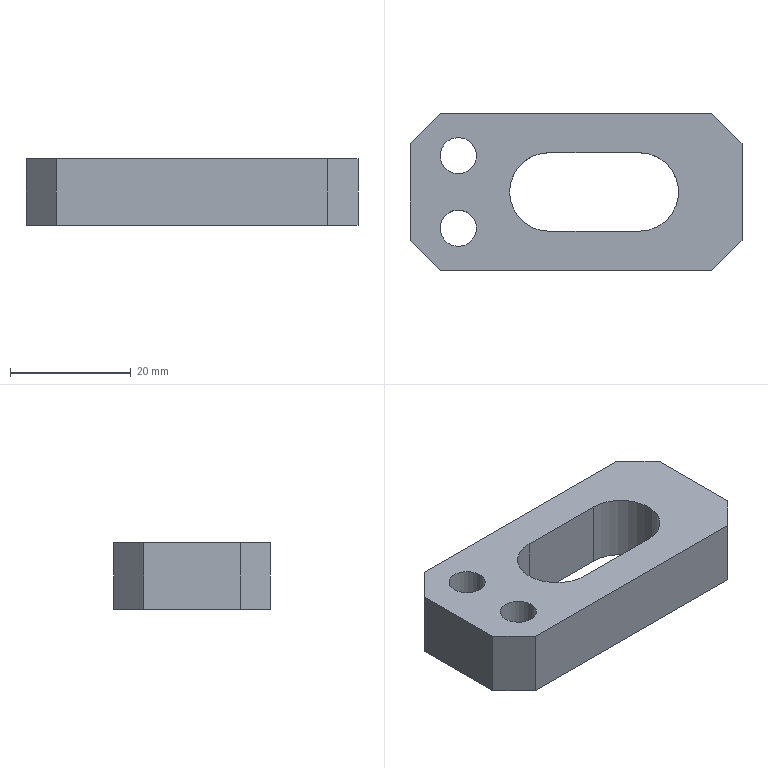Part | SolidWorks | features Chamfer 1, Extrusion 1 | 1 solid | 19 faces | box 55 x 26 x 11 mm | volume 10953 mm3 | plane 12 | cylinder 7 | commonest cylinder face diameters 6 x4 13 x3
STEP:
#1=CARTESIAN_POINT('',(-4.5,6.5,11.));
#2=VERTEX_POINT('',#1);
#3=CARTESIAN_POINT('',(-11.,0.,11.));
#4=VERTEX_POINT('',#3);
#5=CARTESIAN_POINT('',(-4.5,0.,11.));
#6=DIRECTION('',(0.,0.,1.));
#7=DIRECTION('',(1.,0.,0.));
#8=AXIS2_PLACEMENT_3D('',#5,#6,#7);
#9=CIRCLE('',#8,6.5);
#10=EDGE_CURVE('',#2,#4,#9,.T.);
#11=ORIENTED_EDGE('',*,*,#10,.T.);
#12=CARTESIAN_POINT('',(-11.,0.,0.));
#13=VERTEX_POINT('',#12);
#14=CARTESIAN_POINT('',(-11.,0.,11.));
#15=DIRECTION('',(0.,0.,-1.));
#16=VECTOR('',#15,1000.);
#17=LINE('',#14,#16);
#18=EDGE_CURVE('',#4,#13,#17,.T.);
#19=ORIENTED_EDGE('',*,*,#18,.T.);
#20=CARTESIAN_POINT('',(-4.5,6.5,0.));
#21=VERTEX_POINT('',#20);
#22=CARTESIAN_POINT('',(-4.5,0.,0.));
#23=DIRECTION('',(0.,0.,1.));
#24=DIRECTION('',(1.,0.,0.));
#25=AXIS2_PLACEMENT_3D('',#22,#23,#24);
#26=CIRCLE('',#25,6.5);
#27=EDGE_CURVE('',#21,#13,#26,.T.);
#28=ORIENTED_EDGE('',*,*,#27,.F.);
#29=CARTESIAN_POINT('',(-4.5,6.5,11.));
#30=DIRECTION('',(0.,0.,-1.));
#31=VECTOR('',#30,1000.);
#32=LINE('',#29,#31);
#33=EDGE_CURVE('',#2,#21,#32,.T.);
#34=ORIENTED_EDGE('',*,*,#33,.F.);
#35=EDGE_LOOP('',(#11,#19,#28,#34));
#36=FACE_OUTER_BOUND('',#35,.T.);
#37=CARTESIAN_POINT('',(-4.5,0.,11.));
#38=DIRECTION('',(0.,0.,-1.));
#39=DIRECTION('',(-1.,0.,0.));
#40=AXIS2_PLACEMENT_3D('',#37,#38,#39);
#41=CYLINDRICAL_SURFACE('',#40,6.5);
#42=ADVANCED_FACE('',(#36),#41,.F.);
#43=CARTESIAN_POINT('',(-22.5,-6.,11.));
#44=VERTEX_POINT('',#43);
#45=CARTESIAN_POINT('',(-16.5,-6.,11.));
#46=VERTEX_POINT('',#45);
#47=CARTESIAN_POINT('',(-19.5,-6.,11.));
#48=DIRECTION('',(0.,0.,1.));
#49=DIRECTION('',(1.,0.,0.));
#50=AXIS2_PLACEMENT_3D('',#47,#48,#49);
#51=CIRCLE('',#50,3.);
#52=EDGE_CURVE('',#44,#46,#51,.T.);
#53=ORIENTED_EDGE('',*,*,#52,.T.);
#54=CARTESIAN_POINT('',(-16.5,-6.,0.));
#55=VERTEX_POINT('',#54);
#56=CARTESIAN_POINT('',(-16.5,-6.,11.));
#57=DIRECTION('',(0.,0.,-1.));
#58=VECTOR('',#57,1000.);
#59=LINE('',#56,#58);
#60=EDGE_CURVE('',#46,#55,#59,.T.);
#61=ORIENTED_EDGE('',*,*,#60,.T.);
#62=CARTESIAN_POINT('',(-22.5,-6.,0.));
#63=VERTEX_POINT('',#62);
#64=CARTESIAN_POINT('',(-19.5,-6.,0.));
#65=DIRECTION('',(0.,0.,1.));
#66=DIRECTION('',(1.,0.,0.));
#67=AXIS2_PLACEMENT_3D('',#64,#65,#66);
#68=CIRCLE('',#67,3.);
#69=EDGE_CURVE('',#63,#55,#68,.T.);
#70=ORIENTED_EDGE('',*,*,#69,.F.);
#71=CARTESIAN_POINT('',(-22.5,-6.,11.));
#72=DIRECTION('',(0.,0.,-1.));
#73=VECTOR('',#72,1000.);
#74=LINE('',#71,#73);
#75=EDGE_CURVE('',#44,#63,#74,.T.);
#76=ORIENTED_EDGE('',*,*,#75,.F.);
#77=EDGE_LOOP('',(#53,#61,#70,#76));
#78=FACE_OUTER_BOUND('',#77,.T.);
#79=CARTESIAN_POINT('',(-19.5,-6.,11.));
#80=DIRECTION('',(0.,0.,-1.));
#81=DIRECTION('',(-1.,0.,0.));
#82=AXIS2_PLACEMENT_3D('',#79,#80,#81);
#83=CYLINDRICAL_SURFACE('',#82,3.);
#84=ADVANCED_FACE('',(#78),#83,.F.);
#85=CARTESIAN_POINT('',(-22.5,6.,11.));
#86=VERTEX_POINT('',#85);
#87=CARTESIAN_POINT('',(-16.5,6.,11.));
#88=VERTEX_POINT('',#87);
#89=CARTESIAN_POINT('',(-19.5,6.,11.));
#90=DIRECTION('',(0.,0.,1.));
#91=DIRECTION('',(1.,0.,0.));
#92=AXIS2_PLACEMENT_3D('',#89,#90,#91);
#93=CIRCLE('',#92,3.);
#94=EDGE_CURVE('',#86,#88,#93,.T.);
#95=ORIENTED_EDGE('',*,*,#94,.T.);
#96=CARTESIAN_POINT('',(-16.5,6.,0.));
#97=VERTEX_POINT('',#96);
#98=CARTESIAN_POINT('',(-16.5,6.,11.));
#99=DIRECTION('',(0.,0.,-1.));
#100=VECTOR('',#99,1000.);
#101=LINE('',#98,#100);
#102=EDGE_CURVE('',#88,#97,#101,.T.);
#103=ORIENTED_EDGE('',*,*,#102,.T.);
#104=CARTESIAN_POINT('',(-22.5,6.,0.));
#105=VERTEX_POINT('',#104);
#106=CARTESIAN_POINT('',(-19.5,6.,0.));
#107=DIRECTION('',(0.,0.,1.));
#108=DIRECTION('',(1.,0.,0.));
#109=AXIS2_PLACEMENT_3D('',#106,#107,#108);
#110=CIRCLE('',#109,3.);
#111=EDGE_CURVE('',#105,#97,#110,.T.);
#112=ORIENTED_EDGE('',*,*,#111,.F.);
#113=CARTESIAN_POINT('',(-22.5,6.,11.));
#114=DIRECTION('',(0.,0.,-1.));
#115=VECTOR('',#114,1000.);
#116=LINE('',#113,#115);
#117=EDGE_CURVE('',#86,#105,#116,.T.);
#118=ORIENTED_EDGE('',*,*,#117,.F.);
#119=EDGE_LOOP('',(#95,#103,#112,#118));
#120=FACE_OUTER_BOUND('',#119,.T.);
#121=CARTESIAN_POINT('',(-19.5,6.,11.));
#122=DIRECTION('',(0.,0.,-1.));
#123=DIRECTION('',(-1.,0.,0.));
#124=AXIS2_PLACEMENT_3D('',#121,#122,#123);
#125=CYLINDRICAL_SURFACE('',#124,3.);
#126=ADVANCED_FACE('',(#120),#125,.F.);
#127=ORIENTED_EDGE('',*,*,#52,.F.);
#128=CARTESIAN_POINT('',(-19.5,-6.,11.));
#129=DIRECTION('',(0.,0.,1.));
#130=DIRECTION('',(1.,0.,0.));
#131=AXIS2_PLACEMENT_3D('',#128,#129,#130);
#132=CIRCLE('',#131,3.);
#133=EDGE_CURVE('',#46,#44,#132,.T.);
#134=ORIENTED_EDGE('',*,*,#133,.F.);
#135=EDGE_LOOP('',(#127,#134));
#136=FACE_BOUND('',#135,.T.);
#137=ORIENTED_EDGE('',*,*,#94,.F.);
#138=CARTESIAN_POINT('',(-19.5,6.,11.));
#139=DIRECTION('',(0.,0.,1.));
#140=DIRECTION('',(1.,0.,0.));
#141=AXIS2_PLACEMENT_3D('',#138,#139,#140);
#142=CIRCLE('',#141,3.);
#143=EDGE_CURVE('',#88,#86,#142,.T.);
#144=ORIENTED_EDGE('',*,*,#143,.F.);
#145=EDGE_LOOP('',(#137,#144));
#146=FACE_BOUND('',#145,.T.);
#147=CARTESIAN_POINT('',(-22.5,-13.,11.));
#148=VERTEX_POINT('',#147);
#149=CARTESIAN_POINT('',(22.5,-13.,11.));
#150=VERTEX_POINT('',#149);
#151=CARTESIAN_POINT('',(-27.5,-13.,11.));
#152=DIRECTION('',(1.,0.,0.));
#153=VECTOR('',#152,1000.);
#154=LINE('',#151,#153);
#155=EDGE_CURVE('',#148,#150,#154,.T.);
#156=ORIENTED_EDGE('',*,*,#155,.T.);
#157=CARTESIAN_POINT('',(27.5,-8.,11.));
#158=VERTEX_POINT('',#157);
#159=CARTESIAN_POINT('',(27.5,-8.,11.));
#160=DIRECTION('',(0.7071,0.7071,0.));
#161=VECTOR('',#160,1000.);
#162=LINE('',#159,#161);
#163=EDGE_CURVE('',#150,#158,#162,.T.);
#164=ORIENTED_EDGE('',*,*,#163,.T.);
#165=CARTESIAN_POINT('',(27.5,8.,11.));
#166=VERTEX_POINT('',#165);
#167=CARTESIAN_POINT('',(27.5,-13.,11.));
#168=DIRECTION('',(0.,1.,0.));
#169=VECTOR('',#168,1000.);
#170=LINE('',#167,#169);
#171=EDGE_CURVE('',#158,#166,#170,.T.);
#172=ORIENTED_EDGE('',*,*,#171,.T.);
#173=CARTESIAN_POINT('',(22.5,13.,11.));
#174=VERTEX_POINT('',#173);
#175=CARTESIAN_POINT('',(22.5,13.,11.));
#176=DIRECTION('',(-0.7071,0.7071,0.));
#177=VECTOR('',#176,1000.);
#178=LINE('',#175,#177);
#179=EDGE_CURVE('',#166,#174,#178,.T.);
#180=ORIENTED_EDGE('',*,*,#179,.T.);
#181=CARTESIAN_POINT('',(-22.5,13.,11.));
#182=VERTEX_POINT('',#181);
#183=CARTESIAN_POINT('',(-27.5,13.,11.));
#184=DIRECTION('',(-1.,0.,0.));
#185=VECTOR('',#184,1000.);
#186=LINE('',#183,#185);
#187=EDGE_CURVE('',#174,#182,#186,.T.);
#188=ORIENTED_EDGE('',*,*,#187,.T.);
#189=CARTESIAN_POINT('',(-27.5,8.,11.));
#190=VERTEX_POINT('',#189);
#191=CARTESIAN_POINT('',(-27.5,8.,11.));
#192=DIRECTION('',(-0.7071,-0.7071,0.));
#193=VECTOR('',#192,1000.);
#194=LINE('',#191,#193);
#195=EDGE_CURVE('',#182,#190,#194,.T.);
#196=ORIENTED_EDGE('',*,*,#195,.T.);
#197=CARTESIAN_POINT('',(-27.5,-8.,11.));
#198=VERTEX_POINT('',#197);
#199=CARTESIAN_POINT('',(-27.5,-13.,11.));
#200=DIRECTION('',(0.,-1.,0.));
#201=VECTOR('',#200,1000.);
#202=LINE('',#199,#201);
#203=EDGE_CURVE('',#190,#198,#202,.T.);
#204=ORIENTED_EDGE('',*,*,#203,.T.);
#205=CARTESIAN_POINT('',(-22.5,-13.,11.));
#206=DIRECTION('',(0.7071,-0.7071,0.));
#207=VECTOR('',#206,1000.);
#208=LINE('',#205,#207);
#209=EDGE_CURVE('',#198,#148,#208,.T.);
#210=ORIENTED_EDGE('',*,*,#209,.T.);
#211=EDGE_LOOP('',(#156,#164,#172,#180,#188,#196,#204,#210));
#212=FACE_OUTER_BOUND('',#211,.T.);
#213=ORIENTED_EDGE('',*,*,#10,.F.);
#214=CARTESIAN_POINT('',(10.5,6.5,11.));
#215=VERTEX_POINT('',#214);
#216=CARTESIAN_POINT('',(-4.5,6.5,11.));
#217=DIRECTION('',(-1.,0.,0.));
#218=VECTOR('',#217,1000.);
#219=LINE('',#216,#218);
#220=EDGE_CURVE('',#215,#2,#219,.T.);
#221=ORIENTED_EDGE('',*,*,#220,.F.);
#222=CARTESIAN_POINT('',(10.5,-6.5,11.));
#223=VERTEX_POINT('',#222);
#224=CARTESIAN_POINT('',(10.5,0.,11.));
#225=DIRECTION('',(0.,0.,1.));
#226=DIRECTION('',(1.,0.,0.));
#227=AXIS2_PLACEMENT_3D('',#224,#225,#226);
#228=CIRCLE('',#227,6.5);
#229=EDGE_CURVE('',#223,#215,#228,.T.);
#230=ORIENTED_EDGE('',*,*,#229,.F.);
#231=CARTESIAN_POINT('',(-4.5,-6.5,11.));
#232=VERTEX_POINT('',#231);
#233=CARTESIAN_POINT('',(-4.5,-6.5,11.));
#234=DIRECTION('',(1.,0.,0.));
#235=VECTOR('',#234,1000.);
#236=LINE('',#233,#235);
#237=EDGE_CURVE('',#232,#223,#236,.T.);
#238=ORIENTED_EDGE('',*,*,#237,.F.);
#239=CARTESIAN_POINT('',(-4.5,0.,11.));
#240=DIRECTION('',(0.,0.,1.));
#241=DIRECTION('',(1.,0.,0.));
#242=AXIS2_PLACEMENT_3D('',#239,#240,#241);
#243=CIRCLE('',#242,6.5);
#244=EDGE_CURVE('',#4,#232,#243,.T.);
#245=ORIENTED_EDGE('',*,*,#244,.F.);
#246=EDGE_LOOP('',(#213,#221,#230,#238,#245));
#247=FACE_BOUND('',#246,.T.);
#248=CARTESIAN_POINT('',(0.,0.,11.));
#249=DIRECTION('',(0.,0.,-1.));
#250=DIRECTION('',(-1.,0.,0.));
#251=AXIS2_PLACEMENT_3D('',#248,#249,#250);
#252=PLANE('',#251);
#253=ADVANCED_FACE('',(#136,#146,#212,#247),#252,.F.);
#254=ORIENTED_EDGE('',*,*,#111,.T.);
#255=CARTESIAN_POINT('',(-19.5,6.,0.));
#256=DIRECTION('',(0.,0.,1.));
#257=DIRECTION('',(1.,0.,0.));
#258=AXIS2_PLACEMENT_3D('',#255,#256,#257);
#259=CIRCLE('',#258,3.);
#260=EDGE_CURVE('',#97,#105,#259,.T.);
#261=ORIENTED_EDGE('',*,*,#260,.T.);
#262=EDGE_LOOP('',(#254,#261));
#263=FACE_BOUND('',#262,.T.);
#264=CARTESIAN_POINT('',(27.5,-8.,0.));
#265=VERTEX_POINT('',#264);
#266=CARTESIAN_POINT('',(27.5,8.,0.));
#267=VERTEX_POINT('',#266);
#268=CARTESIAN_POINT('',(27.5,-13.,0.));
#269=DIRECTION('',(0.,1.,0.));
#270=VECTOR('',#269,1000.);
#271=LINE('',#268,#270);
#272=EDGE_CURVE('',#265,#267,#271,.T.);
#273=ORIENTED_EDGE('',*,*,#272,.F.);
#274=CARTESIAN_POINT('',(22.5,-13.,0.));
#275=VERTEX_POINT('',#274);
#276=CARTESIAN_POINT('',(17.75,-17.75,0.));
#277=DIRECTION('',(-0.7071,-0.7071,0.));
#278=VECTOR('',#277,1000.);
#279=LINE('',#276,#278);
#280=EDGE_CURVE('',#265,#275,#279,.T.);
#281=ORIENTED_EDGE('',*,*,#280,.T.);
#282=CARTESIAN_POINT('',(-22.5,-13.,0.));
#283=VERTEX_POINT('',#282);
#284=CARTESIAN_POINT('',(-27.5,-13.,0.));
#285=DIRECTION('',(1.,0.,0.));
#286=VECTOR('',#285,1000.);
#287=LINE('',#284,#286);
#288=EDGE_CURVE('',#283,#275,#287,.T.);
#289=ORIENTED_EDGE('',*,*,#288,.F.);
#290=CARTESIAN_POINT('',(-27.5,-8.,0.));
#291=VERTEX_POINT('',#290);
#292=CARTESIAN_POINT('',(-17.75,-17.75,0.));
#293=DIRECTION('',(-0.7071,0.7071,0.));
#294=VECTOR('',#293,1000.);
#295=LINE('',#292,#294);
#296=EDGE_CURVE('',#283,#291,#295,.T.);
#297=ORIENTED_EDGE('',*,*,#296,.T.);
#298=CARTESIAN_POINT('',(-27.5,8.,0.));
#299=VERTEX_POINT('',#298);
#300=CARTESIAN_POINT('',(-27.5,-13.,0.));
#301=DIRECTION('',(0.,-1.,0.));
#302=VECTOR('',#301,1000.);
#303=LINE('',#300,#302);
#304=EDGE_CURVE('',#299,#291,#303,.T.);
#305=ORIENTED_EDGE('',*,*,#304,.F.);
#306=CARTESIAN_POINT('',(-22.5,13.,0.));
#307=VERTEX_POINT('',#306);
#308=CARTESIAN_POINT('',(-17.75,17.75,0.));
#309=DIRECTION('',(0.7071,0.7071,0.));
#310=VECTOR('',#309,1000.);
#311=LINE('',#308,#310);
#312=EDGE_CURVE('',#299,#307,#311,.T.);
#313=ORIENTED_EDGE('',*,*,#312,.T.);
#314=CARTESIAN_POINT('',(22.5,13.,0.));
#315=VERTEX_POINT('',#314);
#316=CARTESIAN_POINT('',(-27.5,13.,0.));
#317=DIRECTION('',(-1.,0.,0.));
#318=VECTOR('',#317,1000.);
#319=LINE('',#316,#318);
#320=EDGE_CURVE('',#315,#307,#319,.T.);
#321=ORIENTED_EDGE('',*,*,#320,.F.);
#322=CARTESIAN_POINT('',(17.75,17.75,0.));
#323=DIRECTION('',(0.7071,-0.7071,0.));
#324=VECTOR('',#323,1000.);
#325=LINE('',#322,#324);
#326=EDGE_CURVE('',#315,#267,#325,.T.);
#327=ORIENTED_EDGE('',*,*,#326,.T.);
#328=EDGE_LOOP('',(#273,#281,#289,#297,#305,#313,#321,#327));
#329=FACE_OUTER_BOUND('',#328,.T.);
#330=ORIENTED_EDGE('',*,*,#69,.T.);
#331=CARTESIAN_POINT('',(-19.5,-6.,0.));
#332=DIRECTION('',(0.,0.,1.));
#333=DIRECTION('',(1.,0.,0.));
#334=AXIS2_PLACEMENT_3D('',#331,#332,#333);
#335=CIRCLE('',#334,3.);
#336=EDGE_CURVE('',#55,#63,#335,.T.);
#337=ORIENTED_EDGE('',*,*,#336,.T.);
#338=EDGE_LOOP('',(#330,#337));
#339=FACE_BOUND('',#338,.T.);
#340=CARTESIAN_POINT('',(10.5,6.5,0.));
#341=VERTEX_POINT('',#340);
#342=CARTESIAN_POINT('',(-4.5,6.5,0.));
#343=DIRECTION('',(-1.,0.,0.));
#344=VECTOR('',#343,1000.);
#345=LINE('',#342,#344);
#346=EDGE_CURVE('',#341,#21,#345,.T.);
#347=ORIENTED_EDGE('',*,*,#346,.T.);
#348=ORIENTED_EDGE('',*,*,#27,.T.);
#349=CARTESIAN_POINT('',(-4.5,-6.5,0.));
#350=VERTEX_POINT('',#349);
#351=CARTESIAN_POINT('',(-4.5,0.,0.));
#352=DIRECTION('',(0.,0.,1.));
#353=DIRECTION('',(1.,0.,0.));
#354=AXIS2_PLACEMENT_3D('',#351,#352,#353);
#355=CIRCLE('',#354,6.5);
#356=EDGE_CURVE('',#13,#350,#355,.T.);
#357=ORIENTED_EDGE('',*,*,#356,.T.);
#358=CARTESIAN_POINT('',(10.5,-6.5,0.));
#359=VERTEX_POINT('',#358);
#360=CARTESIAN_POINT('',(-4.5,-6.5,0.));
#361=DIRECTION('',(1.,0.,0.));
#362=VECTOR('',#361,1000.);
#363=LINE('',#360,#362);
#364=EDGE_CURVE('',#350,#359,#363,.T.);
#365=ORIENTED_EDGE('',*,*,#364,.T.);
#366=CARTESIAN_POINT('',(10.5,0.,0.));
#367=DIRECTION('',(0.,0.,1.));
#368=DIRECTION('',(1.,0.,0.));
#369=AXIS2_PLACEMENT_3D('',#366,#367,#368);
#370=CIRCLE('',#369,6.5);
#371=EDGE_CURVE('',#359,#341,#370,.T.);
#372=ORIENTED_EDGE('',*,*,#371,.T.);
#373=EDGE_LOOP('',(#347,#348,#357,#365,#372));
#374=FACE_BOUND('',#373,.T.);
#375=CARTESIAN_POINT('',(0.,0.,0.));
#376=DIRECTION('',(0.,0.,-1.));
#377=DIRECTION('',(-1.,0.,0.));
#378=AXIS2_PLACEMENT_3D('',#375,#376,#377);
#379=PLANE('',#378);
#380=ADVANCED_FACE('',(#263,#329,#339,#374),#379,.T.);
#381=ORIENTED_EDGE('',*,*,#171,.F.);
#382=CARTESIAN_POINT('',(27.5,-8.,11.));
#383=DIRECTION('',(0.,0.,-1.));
#384=VECTOR('',#383,1000.);
#385=LINE('',#382,#384);
#386=EDGE_CURVE('',#158,#265,#385,.T.);
#387=ORIENTED_EDGE('',*,*,#386,.T.);
#388=ORIENTED_EDGE('',*,*,#272,.T.);
#389=CARTESIAN_POINT('',(27.5,8.,11.));
#390=DIRECTION('',(0.,0.,1.));
#391=VECTOR('',#390,1000.);
#392=LINE('',#389,#391);
#393=EDGE_CURVE('',#267,#166,#392,.T.);
#394=ORIENTED_EDGE('',*,*,#393,.T.);
#395=EDGE_LOOP('',(#381,#387,#388,#394));
#396=FACE_OUTER_BOUND('',#395,.T.);
#397=CARTESIAN_POINT('',(27.5,-13.,11.));
#398=DIRECTION('',(-1.,0.,0.));
#399=DIRECTION('',(0.,0.,1.));
#400=AXIS2_PLACEMENT_3D('',#397,#398,#399);
#401=PLANE('',#400);
#402=ADVANCED_FACE('',(#396),#401,.F.);
#403=ORIENTED_EDGE('',*,*,#187,.F.);
#404=CARTESIAN_POINT('',(22.5,13.,11.));
#405=DIRECTION('',(0.,0.,-1.));
#406=VECTOR('',#405,1000.);
#407=LINE('',#404,#406);
#408=EDGE_CURVE('',#174,#315,#407,.T.);
#409=ORIENTED_EDGE('',*,*,#408,.T.);
#410=ORIENTED_EDGE('',*,*,#320,.T.);
#411=CARTESIAN_POINT('',(-22.5,13.,11.));
#412=DIRECTION('',(0.,0.,1.));
#413=VECTOR('',#412,1000.);
#414=LINE('',#411,#413);
#415=EDGE_CURVE('',#307,#182,#414,.T.);
#416=ORIENTED_EDGE('',*,*,#415,.T.);
#417=EDGE_LOOP('',(#403,#409,#410,#416));
#418=FACE_OUTER_BOUND('',#417,.T.);
#419=CARTESIAN_POINT('',(-27.5,13.,11.));
#420=DIRECTION('',(0.,-1.,0.));
#421=DIRECTION('',(0.,0.,-1.));
#422=AXIS2_PLACEMENT_3D('',#419,#420,#421);
#423=PLANE('',#422);
#424=ADVANCED_FACE('',(#418),#423,.F.);
#425=ORIENTED_EDGE('',*,*,#304,.T.);
#426=CARTESIAN_POINT('',(-27.5,-8.,11.));
#427=DIRECTION('',(0.,0.,1.));
#428=VECTOR('',#427,1000.);
#429=LINE('',#426,#428);
#430=EDGE_CURVE('',#291,#198,#429,.T.);
#431=ORIENTED_EDGE('',*,*,#430,.T.);
#432=ORIENTED_EDGE('',*,*,#203,.F.);
#433=CARTESIAN_POINT('',(-27.5,8.,11.));
#434=DIRECTION('',(0.,0.,-1.));
#435=VECTOR('',#434,1000.);
#436=LINE('',#433,#435);
#437=EDGE_CURVE('',#190,#299,#436,.T.);
#438=ORIENTED_EDGE('',*,*,#437,.T.);
#439=EDGE_LOOP('',(#425,#431,#432,#438));
#440=FACE_OUTER_BOUND('',#439,.T.);
#441=CARTESIAN_POINT('',(-27.5,-13.,11.));
#442=DIRECTION('',(1.,0.,0.));
#443=DIRECTION('',(0.,0.,-1.));
#444=AXIS2_PLACEMENT_3D('',#441,#442,#443);
#445=PLANE('',#444);
#446=ADVANCED_FACE('',(#440),#445,.F.);
#447=ORIENTED_EDGE('',*,*,#288,.T.);
#448=CARTESIAN_POINT('',(22.5,-13.,11.));
#449=DIRECTION('',(0.,0.,1.));
#450=VECTOR('',#449,1000.);
#451=LINE('',#448,#450);
#452=EDGE_CURVE('',#275,#150,#451,.T.);
#453=ORIENTED_EDGE('',*,*,#452,.T.);
#454=ORIENTED_EDGE('',*,*,#155,.F.);
#455=CARTESIAN_POINT('',(-22.5,-13.,11.));
#456=DIRECTION('',(0.,0.,-1.));
#457=VECTOR('',#456,1000.);
#458=LINE('',#455,#457);
#459=EDGE_CURVE('',#148,#283,#458,.T.);
#460=ORIENTED_EDGE('',*,*,#459,.T.);
#461=EDGE_LOOP('',(#447,#453,#454,#460));
#462=FACE_OUTER_BOUND('',#461,.T.);
#463=CARTESIAN_POINT('',(-27.5,-13.,11.));
#464=DIRECTION('',(0.,1.,0.));
#465=DIRECTION('',(0.,0.,1.));
#466=AXIS2_PLACEMENT_3D('',#463,#464,#465);
#467=PLANE('',#466);
#468=ADVANCED_FACE('',(#462),#467,.F.);
#469=ORIENTED_EDGE('',*,*,#102,.F.);
#470=ORIENTED_EDGE('',*,*,#143,.T.);
#471=ORIENTED_EDGE('',*,*,#117,.T.);
#472=ORIENTED_EDGE('',*,*,#260,.F.);
#473=EDGE_LOOP('',(#469,#470,#471,#472));
#474=FACE_OUTER_BOUND('',#473,.T.);
#475=CARTESIAN_POINT('',(-19.5,6.,11.));
#476=DIRECTION('',(0.,0.,-1.));
#477=DIRECTION('',(-1.,0.,0.));
#478=AXIS2_PLACEMENT_3D('',#475,#476,#477);
#479=CYLINDRICAL_SURFACE('',#478,3.);
#480=ADVANCED_FACE('',(#474),#479,.F.);
#481=ORIENTED_EDGE('',*,*,#60,.F.);
#482=ORIENTED_EDGE('',*,*,#133,.T.);
#483=ORIENTED_EDGE('',*,*,#75,.T.);
#484=ORIENTED_EDGE('',*,*,#336,.F.);
#485=EDGE_LOOP('',(#481,#482,#483,#484));
#486=FACE_OUTER_BOUND('',#485,.T.);
#487=CARTESIAN_POINT('',(-19.5,-6.,11.));
#488=DIRECTION('',(0.,0.,-1.));
#489=DIRECTION('',(-1.,0.,0.));
#490=AXIS2_PLACEMENT_3D('',#487,#488,#489);
#491=CYLINDRICAL_SURFACE('',#490,3.);
#492=ADVANCED_FACE('',(#486),#491,.F.);
#493=ORIENTED_EDGE('',*,*,#18,.F.);
#494=ORIENTED_EDGE('',*,*,#244,.T.);
#495=CARTESIAN_POINT('',(-4.5,-6.5,11.));
#496=DIRECTION('',(0.,0.,-1.));
#497=VECTOR('',#496,1000.);
#498=LINE('',#495,#497);
#499=EDGE_CURVE('',#232,#350,#498,.T.);
#500=ORIENTED_EDGE('',*,*,#499,.T.);
#501=ORIENTED_EDGE('',*,*,#356,.F.);
#502=EDGE_LOOP('',(#493,#494,#500,#501));
#503=FACE_OUTER_BOUND('',#502,.T.);
#504=CARTESIAN_POINT('',(-4.5,0.,11.));
#505=DIRECTION('',(0.,0.,-1.));
#506=DIRECTION('',(-1.,0.,0.));
#507=AXIS2_PLACEMENT_3D('',#504,#505,#506);
#508=CYLINDRICAL_SURFACE('',#507,6.5);
#509=ADVANCED_FACE('',(#503),#508,.F.);
#510=ORIENTED_EDGE('',*,*,#364,.F.);
#511=ORIENTED_EDGE('',*,*,#499,.F.);
#512=ORIENTED_EDGE('',*,*,#237,.T.);
#513=CARTESIAN_POINT('',(10.5,-6.5,11.));
#514=DIRECTION('',(0.,0.,-1.));
#515=VECTOR('',#514,1000.);
#516=LINE('',#513,#515);
#517=EDGE_CURVE('',#223,#359,#516,.T.);
#518=ORIENTED_EDGE('',*,*,#517,.T.);
#519=EDGE_LOOP('',(#510,#511,#512,#518));
#520=FACE_OUTER_BOUND('',#519,.T.);
#521=CARTESIAN_POINT('',(-4.5,-6.5,11.));
#522=DIRECTION('',(0.,1.,0.));
#523=DIRECTION('',(0.,0.,1.));
#524=AXIS2_PLACEMENT_3D('',#521,#522,#523);
#525=PLANE('',#524);
#526=ADVANCED_FACE('',(#520),#525,.T.);
#527=ORIENTED_EDGE('',*,*,#371,.F.);
#528=ORIENTED_EDGE('',*,*,#517,.F.);
#529=ORIENTED_EDGE('',*,*,#229,.T.);
#530=CARTESIAN_POINT('',(10.5,6.5,11.));
#531=DIRECTION('',(0.,0.,-1.));
#532=VECTOR('',#531,1000.);
#533=LINE('',#530,#532);
#534=EDGE_CURVE('',#215,#341,#533,.T.);
#535=ORIENTED_EDGE('',*,*,#534,.T.);
#536=EDGE_LOOP('',(#527,#528,#529,#535));
#537=FACE_OUTER_BOUND('',#536,.T.);
#538=CARTESIAN_POINT('',(10.5,0.,11.));
#539=DIRECTION('',(0.,0.,-1.));
#540=DIRECTION('',(-1.,0.,0.));
#541=AXIS2_PLACEMENT_3D('',#538,#539,#540);
#542=CYLINDRICAL_SURFACE('',#541,6.5);
#543=ADVANCED_FACE('',(#537),#542,.F.);
#544=ORIENTED_EDGE('',*,*,#346,.F.);
#545=ORIENTED_EDGE('',*,*,#534,.F.);
#546=ORIENTED_EDGE('',*,*,#220,.T.);
#547=ORIENTED_EDGE('',*,*,#33,.T.);
#548=EDGE_LOOP('',(#544,#545,#546,#547));
#549=FACE_OUTER_BOUND('',#548,.T.);
#550=CARTESIAN_POINT('',(-4.5,6.5,11.));
#551=DIRECTION('',(0.,-1.,0.));
#552=DIRECTION('',(0.,0.,-1.));
#553=AXIS2_PLACEMENT_3D('',#550,#551,#552);
#554=PLANE('',#553);
#555=ADVANCED_FACE('',(#549),#554,.T.);
#556=ORIENTED_EDGE('',*,*,#163,.F.);
#557=ORIENTED_EDGE('',*,*,#452,.F.);
#558=ORIENTED_EDGE('',*,*,#280,.F.);
#559=ORIENTED_EDGE('',*,*,#386,.F.);
#560=EDGE_LOOP('',(#556,#557,#558,#559));
#561=FACE_OUTER_BOUND('',#560,.T.);
#562=CARTESIAN_POINT('',(27.5,-8.,11.));
#563=DIRECTION('',(-0.7071,0.7071,0.));
#564=DIRECTION('',(0.,0.,-1.));
#565=AXIS2_PLACEMENT_3D('',#562,#563,#564);
#566=PLANE('',#565);
#567=ADVANCED_FACE('',(#561),#566,.F.);
#568=ORIENTED_EDGE('',*,*,#179,.F.);
#569=ORIENTED_EDGE('',*,*,#393,.F.);
#570=ORIENTED_EDGE('',*,*,#326,.F.);
#571=ORIENTED_EDGE('',*,*,#408,.F.);
#572=EDGE_LOOP('',(#568,#569,#570,#571));
#573=FACE_OUTER_BOUND('',#572,.T.);
#574=CARTESIAN_POINT('',(22.5,13.,11.));
#575=DIRECTION('',(-0.7071,-0.7071,0.));
#576=DIRECTION('',(0.,0.,-1.));
#577=AXIS2_PLACEMENT_3D('',#574,#575,#576);
#578=PLANE('',#577);
#579=ADVANCED_FACE('',(#573),#578,.F.);
#580=ORIENTED_EDGE('',*,*,#209,.F.);
#581=ORIENTED_EDGE('',*,*,#430,.F.);
#582=ORIENTED_EDGE('',*,*,#296,.F.);
#583=ORIENTED_EDGE('',*,*,#459,.F.);
#584=EDGE_LOOP('',(#580,#581,#582,#583));
#585=FACE_OUTER_BOUND('',#584,.T.);
#586=CARTESIAN_POINT('',(-22.5,-13.,11.));
#587=DIRECTION('',(0.7071,0.7071,0.));
#588=DIRECTION('',(0.,0.,-1.));
#589=AXIS2_PLACEMENT_3D('',#586,#587,#588);
#590=PLANE('',#589);
#591=ADVANCED_FACE('',(#585),#590,.F.);
#592=ORIENTED_EDGE('',*,*,#195,.F.);
#593=ORIENTED_EDGE('',*,*,#415,.F.);
#594=ORIENTED_EDGE('',*,*,#312,.F.);
#595=ORIENTED_EDGE('',*,*,#437,.F.);
#596=EDGE_LOOP('',(#592,#593,#594,#595));
#597=FACE_OUTER_BOUND('',#596,.T.);
#598=CARTESIAN_POINT('',(-27.5,8.,11.));
#599=DIRECTION('',(0.7071,-0.7071,0.));
#600=DIRECTION('',(0.,0.,-1.));
#601=AXIS2_PLACEMENT_3D('',#598,#599,#600);
#602=PLANE('',#601);
#603=ADVANCED_FACE('',(#597),#602,.F.);
#604=CLOSED_SHELL('',(#42,#84,#126,#253,#380,#402,#424,#446,#468,#480,#492,#509,#526,#543,#555,#567,#579,#591,#603));
#605=MANIFOLD_SOLID_BREP('',#604);
#606=CARTESIAN_POINT('',(0.,0.,0.));
#607=DIRECTION('',(0.,0.,1.));
#608=DIRECTION('',(1.,0.,0.));
#609=AXIS2_PLACEMENT_3D('',#606,#607,#608);
#610=(LENGTH_UNIT()NAMED_UNIT(*)SI_UNIT(.MILLI.,.METRE.));
#611=UNCERTAINTY_MEASURE_WITH_UNIT(LENGTH_MEASURE(0.00001),#610,'','');
#612=(NAMED_UNIT(*)PLANE_ANGLE_UNIT()SI_UNIT($,.RADIAN.));
#613=(NAMED_UNIT(*)SI_UNIT($,.STERADIAN.)SOLID_ANGLE_UNIT());
#614=(GEOMETRIC_REPRESENTATION_CONTEXT(3)GLOBAL_UNCERTAINTY_ASSIGNED_CONTEXT((#611))GLOBAL_UNIT_ASSIGNED_CONTEXT((#610,#612,#613))REPRESENTATION_CONTEXT('',''));
#615=ADVANCED_BREP_SHAPE_REPRESENTATION('',(#605,#609),#614);